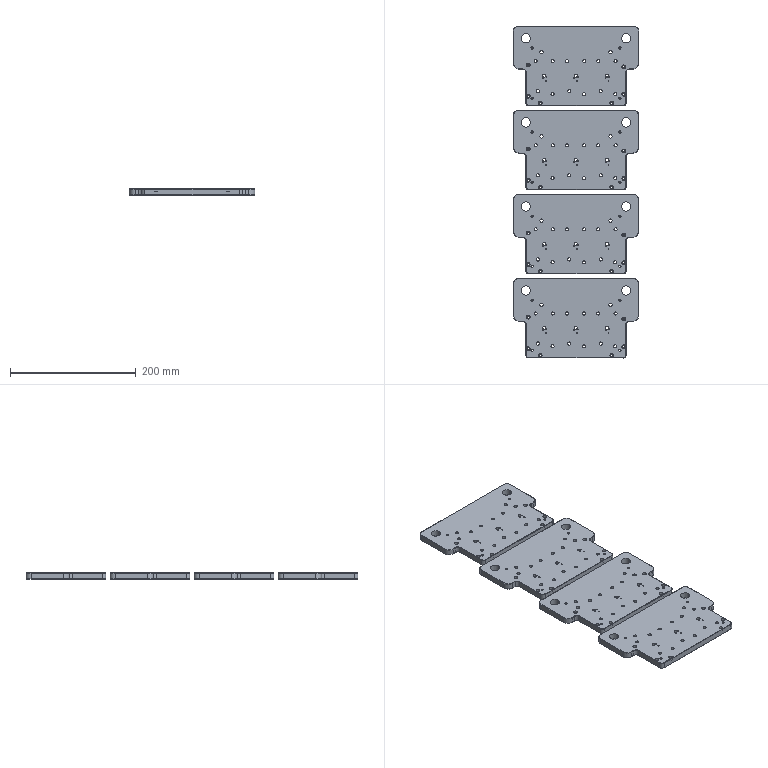NC program | NX | posted with a generic post | part box 200 x 529 x 10 mm
Lines 1 to 1503 of 1801, first 1182 of 1477 lines:
N10 G17 G21 G94 G90
(DRILLING_COPY , TOOL : D4A45)
N12 T02 M6
N14 G54
N16 G17 G0 G90 X80. Y44. S5000 M3
N18 G43 Z30. H2
N20 G94 G81 G98 Z-0.6 F250. R3.
N22 X70. Y28.5
N24 X55. Y21.5
N26 X64.397 Y7.41
N28 X76. Y1.5
N30 X60.727 Y-40.475
N32 X76. Y-48.5
N34 X70. Y-51.5
N36 X57. Y-59.5
N38 X37.379 Y-45.039
N40 X48.194 Y-24.555
N42 Y-23.158
N44 X52.858 Y-18.927
N46 X50.608 Y-15.627
N48 X47.178 Y-17.697
N50 X36.956 Y7.4
N52 X14.397 Y7.41
N54 X-13.044 Y7.4
N56 X-2.822 Y-17.697
N58 X0.608 Y-15.627
N60 X2.858 Y-18.927
N62 X-1.806 Y-23.158
N64 Y-24.555
N66 X10.727 Y-40.475
N68 X-12.621 Y-45.039
N70 X-39.273 Y-40.475
N72 X-57. Y-59.5
N74 X-70. Y-51.5
N76 X-76. Y-45.5
N78 X-62.621 Y-45.039
N80 X-51.806 Y-24.555
N82 Y-23.158
N84 X-47.142 Y-18.927
N86 X-49.392 Y-15.627
N88 X-52.822 Y-17.697
N90 X-76. Y-1.5
N92 X-63.044 Y7.4
N94 X-35.603 Y7.41
N96 X-55. Y21.5
N98 X-70. Y28.5
N100 X-80. Y44.
N102 G80
N104 G0 X-80. Y44. Z30.
N106 M5
(DRILLING_COPY_COPY_COPY_COPY_COPY_COPY , TOOL : 1.7ZT)
N108 T17 M6
N110 G54
N112 G17 G0 G90 X-47.142 Y-18.927 S2000 M3
N114 G43 Z30. H17
N116 G94 G83 G98 Z-12.011 F120. Q2. R3.
N118 X2.858
N120 X52.858
N122 G80
N124 G0 X52.858 Y-18.927 Z30.
N126 M5
(DRILLING_COPY_COPY_COPY_COPY_COPY_COPY_COPY , TOOL : 0.97ZT)
N128 T19 M6
N130 G54
N132 G17 G0 G90 X-52.822 Y-17.697 S2000 M3
N134 G43 Z30. H19
N136 G94 G83 G98 Z-11.791 F100. Q2. R3.
N138 X-51.806 Y-23.158
N140 Y-24.555
N142 X-2.822 Y-17.697
N144 X-1.806 Y-23.158
N146 Y-24.555
N148 X47.178 Y-17.697
N150 X48.194 Y-23.158
N152 Y-24.555
N154 G80
N156 G0 X48.194 Y-24.555 Z30.
N158 M5
(DRILLING_COPY_COPY_COPY_COPY_COPY , TOOL : 3.5ZT)
N160 T15 M6
N162 G54
N164 G17 G0 G90 X76. Y1.5 S1910 M3
N166 G43 Z30. H15
N168 G94 G83 G98 Z-8.552 F180. Q2. R3.
N170 Y-48.5
N172 X57. Y-59.5
N174 X-57.
N176 X-76. Y-45.5
N178 Y-1.5
N180 G80
N182 G0 X-76. Y-1.5 Z30.
(DRILLING_COPY_COPY_COPY_COPY_COPY_COPY_1 , TOOL : 3.5ZT)
N184 X-70. Y28.5
N186 G83 Z-12.552 F180. Q2. R3.
N188 Y-51.5
N190 X70.
N192 Y28.5
N194 G80
N196 G0 X70. Y28.5 Z30.
(DRILLING_COPY_COPY_COPY_COPY_COPY_COPY_1_COPY , TOOL : 3.5ZT)
N198 X-12.621 Y-45.039
N200 G83 Z-12.552 F180. Q2. R3.
N202 X10.727 Y-40.475
N204 X37.379 Y-45.039
N206 X60.727 Y-40.475
N208 X50.608 Y-15.627
N210 X64.397 Y7.41
N212 X55. Y21.5
N214 X36.956 Y7.4
N216 X14.397 Y7.41
N218 X0.608 Y-15.627
N220 X-13.044 Y7.4
N222 X-35.603 Y7.41
N224 X-55. Y21.5
N226 X-63.044 Y7.4
N228 X-49.392 Y-15.627
N230 X-39.273 Y-40.475
N232 X-62.621 Y-45.039
N234 G80
N236 G0 X-62.621 Y-45.039 Z30.
N238 M5
(HOLE_MILLING_COPY , TOOL : D4)
N240 T04 M6
N242 G54
N244 G17 G0 G90 X-70. Y28.5 S9500 M3
N246 G43 Z30. H4
N248 Z0.5
N250 G94 G3 X-70.625 Y29.125 R0.625 F2200.
N252 X-71.25 Y28.5 R0.625
N254 X-71.25 Y28.5 Z0.1 I1.25 J0.
N256 X-71.25 Y28.5 Z-0.3 I1.25 J0.
N258 X-71.25 Y28.5 Z-0.7 I1.25 J0.
N260 X-71.25 Y28.5 Z-1.1 I1.25 J0.
N262 X-71.25 Y28.5 Z-1.5 I1.25 J0.
N264 X-71.25 Y28.5 Z-1.9 I1.25 J0.
N266 X-71.25 Y28.5 Z-2.3 I1.25 J0.
N268 X-71.25 Y28.5 Z-2.7 I1.25 J0.
N270 X-71.25 Y28.5 Z-3.1 I1.25 J0.
N272 X-71.25 Y28.5 Z-3.5 I1.25 J0.
N274 X-71.25 Y28.5 Z-3.9 I1.25 J0.
N276 X-70. Y27.25 Z-4. R1.25
N278 X-68.75 Y28.5 R1.25
N280 X-70. Y27.25 R-1.25
N282 X-69.375 Y27.875 R0.625
N284 X-70. Y28.5 R0.625
N286 G0 Z30.
N288 X-55. Y21.5
N290 Z0.5
N292 G3 X-55.5 Y22. R0.5
N294 X-56. Y21.5 R0.5
N296 X-56. Y21.5 Z0.1 I1. J0.
N298 X-56. Y21.5 Z-0.3 I1. J0.
N300 X-56. Y21.5 Z-0.7 I1. J0.
N302 X-56. Y21.5 Z-1.1 I1. J0.
N304 X-56. Y21.5 Z-1.5 I1. J0.
N306 X-56. Y21.5 Z-1.9 I1. J0.
N308 X-55. Y20.5 Z-2. R1.
N310 X-54. Y21.5 R1.
N312 X-55. Y20.5 R-1.
N314 X-54.5 Y21. R0.5
N316 X-55. Y21.5 R0.5
N318 G0 Z30.
N320 X-70. Y-51.5
N322 Z0.5
N324 G3 X-70.625 Y-50.875 R0.625
N326 X-71.25 Y-51.5 R0.625
N328 X-71.25 Y-51.5 Z0.1 I1.25 J0.
N330 X-71.25 Y-51.5 Z-0.3 I1.25 J0.
N332 X-71.25 Y-51.5 Z-0.7 I1.25 J0.
N334 X-71.25 Y-51.5 Z-1.1 I1.25 J0.
N336 X-71.25 Y-51.5 Z-1.5 I1.25 J0.
N338 X-71.25 Y-51.5 Z-1.9 I1.25 J0.
N340 X-71.25 Y-51.5 Z-2.3 I1.25 J0.
N342 X-71.25 Y-51.5 Z-2.7 I1.25 J0.
N344 X-71.25 Y-51.5 Z-3.1 I1.25 J0.
N346 X-71.25 Y-51.5 Z-3.5 I1.25 J0.
N348 X-71.25 Y-51.5 Z-3.9 I1.25 J0.
N350 X-70. Y-52.75 Z-4. R1.25
N352 X-68.75 Y-51.5 R1.25
N354 X-70. Y-52.75 R-1.25
N356 X-69.375 Y-52.125 R0.625
N358 X-70. Y-51.5 R0.625
N360 G0 Z30.
N362 X70.
N364 Z0.5
N366 G3 X69.375 Y-50.875 R0.625
N368 X68.75 Y-51.5 R0.625
N370 X68.75 Y-51.5 Z0.1 I1.25 J0.
N372 X68.75 Y-51.5 Z-0.3 I1.25 J0.
N374 X68.75 Y-51.5 Z-0.7 I1.25 J0.
N376 X68.75 Y-51.5 Z-1.1 I1.25 J0.
N378 X68.75 Y-51.5 Z-1.5 I1.25 J0.
N380 X68.75 Y-51.5 Z-1.9 I1.25 J0.
N382 X68.75 Y-51.5 Z-2.3 I1.25 J0.
N384 X68.75 Y-51.5 Z-2.7 I1.25 J0.
N386 X68.75 Y-51.5 Z-3.1 I1.25 J0.
N388 X68.75 Y-51.5 Z-3.5 I1.25 J0.
N390 X68.75 Y-51.5 Z-3.9 I1.25 J0.
N392 X70. Y-52.75 Z-4. R1.25
N394 X71.25 Y-51.5 R1.25
N396 X70. Y-52.75 R-1.25
N398 X70.625 Y-52.125 R0.625
N400 X70. Y-51.5 R0.625
N402 G0 Z30.
N404 Y28.5
N406 Z0.5
N408 G3 X69.375 Y29.125 R0.625
N410 X68.75 Y28.5 R0.625
N412 X68.75 Y28.5 Z0.1 I1.25 J0.
N414 X68.75 Y28.5 Z-0.3 I1.25 J0.
N416 X68.75 Y28.5 Z-0.7 I1.25 J0.
N418 X68.75 Y28.5 Z-1.1 I1.25 J0.
N420 X68.75 Y28.5 Z-1.5 I1.25 J0.
N422 X68.75 Y28.5 Z-1.9 I1.25 J0.
N424 X68.75 Y28.5 Z-2.3 I1.25 J0.
N426 X68.75 Y28.5 Z-2.7 I1.25 J0.
N428 X68.75 Y28.5 Z-3.1 I1.25 J0.
N430 X68.75 Y28.5 Z-3.5 I1.25 J0.
N432 X68.75 Y28.5 Z-3.9 I1.25 J0.
N434 X70. Y27.25 Z-4. R1.25
N436 X71.25 Y28.5 R1.25
N438 X70. Y27.25 R-1.25
N440 X70.625 Y27.875 R0.625
N442 X70. Y28.5 R0.625
N444 G0 Z30.
N446 X55. Y21.5
N448 Z0.5
N450 G3 X54.5 Y22. R0.5
N452 X54. Y21.5 R0.5
N454 X54. Y21.5 Z0.1 I1. J0.
N456 X54. Y21.5 Z-0.3 I1. J0.
N458 X54. Y21.5 Z-0.7 I1. J0.
N460 X54. Y21.5 Z-1.1 I1. J0.
N462 X54. Y21.5 Z-1.5 I1. J0.
N464 X54. Y21.5 Z-1.9 I1. J0.
N466 X55. Y20.5 Z-2. R1.
N468 X56. Y21.5 R1.
N470 X55. Y20.5 R-1.
N472 X55.5 Y21. R0.5
N474 X55. Y21.5 R0.5
N476 G0 Z30.
N478 M5
(HOLE_MILLING_1 , TOOL : D6)
N480 T06 M6
N482 G54
N484 G17 G0 G90 X-80. Y44. S9500 M3
N486 G43 Z30. H6
N488 Z0.5
N490 G94 G3 X-81.1 Y45.1 R1.1 F2200.
N492 X-82.2 Y44. R1.1
N494 X-82.2 Y44. Z0. I2.2 J0.
N496 X-82.2 Y44. Z-0.5 I2.2 J0.
N498 X-82.2 Y44. Z-1. I2.2 J0.
N500 X-82.2 Y44. Z-1.5 I2.2 J0.
N502 X-82.2 Y44. Z-2. I2.2 J0.
N504 X-82.2 Y44. Z-2.5 I2.2 J0.
N506 X-82.2 Y44. Z-3. I2.2 J0.
N508 X-82.2 Y44. Z-3.5 I2.2 J0.
N510 X-82.2 Y44. Z-4. I2.2 J0.
N512 X-82.2 Y44. Z-4.5 I2.2 J0.
N514 X-82.2 Y44. Z-5. I2.2 J0.
N516 X-82.2 Y44. Z-5.5 I2.2 J0.
N518 X-82.2 Y44. Z-6. I2.2 J0.
N520 X-82.2 Y44. Z-6.5 I2.2 J0.
N522 X-82.2 Y44. Z-7. I2.2 J0.
N524 X-82.2 Y44. Z-7.5 I2.2 J0.
N526 X-82.2 Y44. Z-8. I2.2 J0.
N528 X-82.2 Y44. Z-8.5 I2.2 J0.
N530 X-82.2 Y44. Z-9. I2.2 J0.
N532 X-82.2 Y44. Z-9.5 I2.2 J0.
N534 X-82.2 Y44. Z-10. I2.2 J0.
N536 X-80. Y41.8 R2.2
N538 X-82.2 Y44. R-2.2
N540 X-81.1 Y42.9 R1.1
N542 X-80. Y44. R1.1
N544 G0 Z0.5
N546 G3 X-82.2 Y46.2 R2.2
N548 X-84.4 Y44. R2.2
N550 X-84.4 Y44. Z0. I4.4 J0.
N552 X-84.4 Y44. Z-0.5 I4.4 J0.
N554 X-84.4 Y44. Z-1. I4.4 J0.
N556 X-84.4 Y44. Z-1.5 I4.4 J0.
N558 X-84.4 Y44. Z-2. I4.4 J0.
N560 X-84.4 Y44. Z-2.5 I4.4 J0.
N562 X-84.4 Y44. Z-3. I4.4 J0.
N564 X-84.4 Y44. Z-3.5 I4.4 J0.
N566 X-84.4 Y44. Z-4. I4.4 J0.
N568 X-84.4 Y44. Z-4.5 I4.4 J0.
N570 X-84.4 Y44. Z-5. I4.4 J0.
N572 X-84.4 Y44. Z-5.5 I4.4 J0.
N574 X-84.4 Y44. Z-6. I4.4 J0.
N576 X-84.4 Y44. Z-6.5 I4.4 J0.
N578 X-84.4 Y44. Z-7. I4.4 J0.
N580 X-84.4 Y44. Z-7.5 I4.4 J0.
N582 X-84.4 Y44. Z-8. I4.4 J0.
N584 X-84.4 Y44. Z-8.5 I4.4 J0.
N586 X-84.4 Y44. Z-9. I4.4 J0.
N588 X-84.4 Y44. Z-9.5 I4.4 J0.
N590 X-84.4 Y44. Z-10. I4.4 J0.
N592 X-80. Y39.6 R4.4
N594 X-84.4 Y44. R-4.4
N596 X-82.2 Y41.8 R2.2
N598 X-80. Y44. R2.2
N600 G0 Z30.
N602 X80.
N604 Z0.5
N606 G3 X78.9 Y45.1 R1.1
N608 X77.8 Y44. R1.1
N610 X77.8 Y44. Z0. I2.2 J0.
N612 X77.8 Y44. Z-0.5 I2.2 J0.
N614 X77.8 Y44. Z-1. I2.2 J0.
N616 X77.8 Y44. Z-1.5 I2.2 J0.
N618 X77.8 Y44. Z-2. I2.2 J0.
N620 X77.8 Y44. Z-2.5 I2.2 J0.
N622 X77.8 Y44. Z-3. I2.2 J0.
N624 X77.8 Y44. Z-3.5 I2.2 J0.
N626 X77.8 Y44. Z-4. I2.2 J0.
N628 X77.8 Y44. Z-4.5 I2.2 J0.
N630 X77.8 Y44. Z-5. I2.2 J0.
N632 X77.8 Y44. Z-5.5 I2.2 J0.
N634 X77.8 Y44. Z-6. I2.2 J0.
N636 X77.8 Y44. Z-6.5 I2.2 J0.
N638 X77.8 Y44. Z-7. I2.2 J0.
N640 X77.8 Y44. Z-7.5 I2.2 J0.
N642 X77.8 Y44. Z-8. I2.2 J0.
N644 X77.8 Y44. Z-8.5 I2.2 J0.
N646 X77.8 Y44. Z-9. I2.2 J0.
N648 X77.8 Y44. Z-9.5 I2.2 J0.
N650 X77.8 Y44. Z-10. I2.2 J0.
N652 X80. Y41.8 R2.2
N654 X77.8 Y44. R-2.2
N656 X78.9 Y42.9 R1.1
N658 X80. Y44. R1.1
N660 G0 Z0.5
N662 G3 X77.8 Y46.2 R2.2
N664 X75.6 Y44. R2.2
N666 X75.6 Y44. Z0. I4.4 J0.
N668 X75.6 Y44. Z-0.5 I4.4 J0.
N670 X75.6 Y44. Z-1. I4.4 J0.
N672 X75.6 Y44. Z-1.5 I4.4 J0.
N674 X75.6 Y44. Z-2. I4.4 J0.
N676 X75.6 Y44. Z-2.5 I4.4 J0.
N678 X75.6 Y44. Z-3. I4.4 J0.
N680 X75.6 Y44. Z-3.5 I4.4 J0.
N682 X75.6 Y44. Z-4. I4.4 J0.
N684 X75.6 Y44. Z-4.5 I4.4 J0.
N686 X75.6 Y44. Z-5. I4.4 J0.
N688 X75.6 Y44. Z-5.5 I4.4 J0.
N690 X75.6 Y44. Z-6. I4.4 J0.
N692 X75.6 Y44. Z-6.5 I4.4 J0.
N694 X75.6 Y44. Z-7. I4.4 J0.
N696 X75.6 Y44. Z-7.5 I4.4 J0.
N698 X75.6 Y44. Z-8. I4.4 J0.
N700 X75.6 Y44. Z-8.5 I4.4 J0.
N702 X75.6 Y44. Z-9. I4.4 J0.
N704 X75.6 Y44. Z-9.5 I4.4 J0.
N706 X75.6 Y44. Z-10. I4.4 J0.
N708 X80. Y39.6 R4.4
N710 X75.6 Y44. R-4.4
N712 X77.8 Y41.8 R2.2
N714 X80. Y44. R2.2
N716 G0 Z30.
N718 M5
(HOLE_MILLING_COPY_COPY , TOOL : D3)
N720 T03 M6
N722 G54
N724 G17 G0 G90 X-63.044 Y7.4 S9500 M3
N726 G43 Z30. H3
N728 Z0.5
N730 G94 G3 X-63.494 Y7.85 R0.45 F1000.
N732 X-63.944 Y7.4 R0.45
N734 X-63.944 Y7.4 Z0.2 I0.9 J0.
N736 X-63.944 Y7.4 Z-0.1 I0.9 J0.
N738 X-63.944 Y7.4 Z-0.4 I0.9 J0.
N740 X-63.944 Y7.4 Z-0.7 I0.9 J0.
N742 X-63.944 Y7.4 Z-1. I0.9 J0.
N744 X-63.944 Y7.4 Z-1.3 I0.9 J0.
N746 X-63.944 Y7.4 Z-1.6 I0.9 J0.
N748 X-63.944 Y7.4 Z-1.9 I0.9 J0.
N750 X-63.944 Y7.4 Z-2.2 I0.9 J0.
N752 X-63.944 Y7.4 Z-2.5 I0.9 J0.
N754 X-63.944 Y7.4 Z-2.8 I0.9 J0.
N756 X-63.944 Y7.4 Z-3.1 I0.9 J0.
N758 X-63.944 Y7.4 Z-3.4 I0.9 J0.
N760 X-63.944 Y7.4 Z-3.7 I0.9 J0.
N762 X-63.944 Y7.4 Z-4. I0.9 J0.
N764 X-63.944 Y7.4 Z-4.3 I0.9 J0.
N766 X-63.944 Y7.4 Z-4.6 I0.9 J0.
N768 X-63.944 Y7.4 Z-4.9 I0.9 J0.
N770 X-63.944 Y7.4 Z-5.2 I0.9 J0.
N772 X-63.944 Y7.4 Z-5.5 I0.9 J0.
N774 X-63.944 Y7.4 Z-5.8 I0.9 J0.
N776 X-63.944 Y7.4 Z-6.1 I0.9 J0.
N778 X-63.944 Y7.4 Z-6.4 I0.9 J0.
N780 X-63.944 Y7.4 Z-6.7 I0.9 J0.
N782 X-63.944 Y7.4 Z-7. I0.9 J0.
N784 X-63.944 Y7.4 Z-7.3 I0.9 J0.
N786 X-63.944 Y7.4 Z-7.6 I0.9 J0.
N788 X-63.944 Y7.4 Z-7.9 I0.9 J0.
N790 X-63.944 Y7.4 Z-8.2 I0.9 J0.
N792 X-63.944 Y7.4 Z-8.5 I0.9 J0.
N794 X-63.944 Y7.4 Z-8.8 I0.9 J0.
N796 X-63.944 Y7.4 Z-9.1 I0.9 J0.
N798 X-63.944 Y7.4 Z-9.4 I0.9 J0.
N800 X-63.944 Y7.4 Z-9.7 I0.9 J0.
N802 X-63.944 Y7.4 Z-10. I0.9 J0.
N804 X-63.044 Y6.5 R0.9
N806 X-63.944 Y7.4 R-0.9
N808 X-63.494 Y6.95 R0.45
N810 X-63.044 Y7.4 R0.45
N812 G0 Z30.
N814 X-49.392 Y-15.627
N816 Z0.5
N818 G3 X-49.842 Y-15.177 R0.45
N820 X-50.292 Y-15.627 R0.45
N822 X-50.292 Y-15.627 Z0.2 I0.9 J0.
N824 X-50.292 Y-15.627 Z-0.1 I0.9 J0.
N826 X-50.292 Y-15.627 Z-0.4 I0.9 J0.
N828 X-50.292 Y-15.627 Z-0.7 I0.9 J0.
N830 X-50.292 Y-15.627 Z-1. I0.9 J0.
N832 X-50.292 Y-15.627 Z-1.3 I0.9 J0.
N834 X-50.292 Y-15.627 Z-1.6 I0.9 J0.
N836 X-50.292 Y-15.627 Z-1.9 I0.9 J0.
N838 X-50.292 Y-15.627 Z-2.2 I0.9 J0.
N840 X-50.292 Y-15.627 Z-2.5 I0.9 J0.
N842 X-50.292 Y-15.627 Z-2.8 I0.9 J0.
N844 X-50.292 Y-15.627 Z-3.1 I0.9 J0.
N846 X-50.292 Y-15.627 Z-3.4 I0.9 J0.
N848 X-50.292 Y-15.627 Z-3.7 I0.9 J0.
N850 X-50.292 Y-15.627 Z-4. I0.9 J0.
N852 X-50.292 Y-15.627 Z-4.3 I0.9 J0.
N854 X-50.292 Y-15.627 Z-4.6 I0.9 J0.
N856 X-50.292 Y-15.627 Z-4.9 I0.9 J0.
N858 X-50.292 Y-15.627 Z-5.2 I0.9 J0.
N860 X-50.292 Y-15.627 Z-5.5 I0.9 J0.
N862 X-50.292 Y-15.627 Z-5.8 I0.9 J0.
N864 X-50.292 Y-15.627 Z-6.1 I0.9 J0.
N866 X-50.292 Y-15.627 Z-6.4 I0.9 J0.
N868 X-50.292 Y-15.627 Z-6.7 I0.9 J0.
N870 X-50.292 Y-15.627 Z-7. I0.9 J0.
N872 X-50.292 Y-15.627 Z-7.3 I0.9 J0.
N874 X-50.292 Y-15.627 Z-7.6 I0.9 J0.
N876 X-50.292 Y-15.627 Z-7.9 I0.9 J0.
N878 X-50.292 Y-15.627 Z-8.2 I0.9 J0.
N880 X-50.292 Y-15.627 Z-8.5 I0.9 J0.
N882 X-50.292 Y-15.627 Z-8.8 I0.9 J0.
N884 X-50.292 Y-15.627 Z-9.1 I0.9 J0.
N886 X-50.292 Y-15.627 Z-9.4 I0.9 J0.
N888 X-50.292 Y-15.627 Z-9.7 I0.9 J0.
N890 X-50.292 Y-15.627 Z-10. I0.9 J0.
N892 X-49.392 Y-16.527 R0.9
N894 X-50.292 Y-15.627 R-0.9
N896 X-49.842 Y-16.077 R0.45
N898 X-49.392 Y-15.627 R0.45
N900 G0 Z30.
N902 X-35.603 Y7.41
N904 Z0.5
N906 G3 X-36.053 Y7.86 R0.45
N908 X-36.503 Y7.41 R0.45
N910 X-36.503 Y7.41 Z0.2 I0.9 J0.
N912 X-36.503 Y7.41 Z-0.1 I0.9 J0.
N914 X-36.503 Y7.41 Z-0.4 I0.9 J0.
N916 X-36.503 Y7.41 Z-0.7 I0.9 J0.
N918 X-36.503 Y7.41 Z-1. I0.9 J0.
N920 X-36.503 Y7.41 Z-1.3 I0.9 J0.
N922 X-36.503 Y7.41 Z-1.6 I0.9 J0.
N924 X-36.503 Y7.41 Z-1.9 I0.9 J0.
N926 X-36.503 Y7.41 Z-2.2 I0.9 J0.
N928 X-36.503 Y7.41 Z-2.5 I0.9 J0.
N930 X-36.503 Y7.41 Z-2.8 I0.9 J0.
N932 X-36.503 Y7.41 Z-3.1 I0.9 J0.
N934 X-36.503 Y7.41 Z-3.4 I0.9 J0.
N936 X-36.503 Y7.41 Z-3.7 I0.9 J0.
N938 X-36.503 Y7.41 Z-4. I0.9 J0.
N940 X-36.503 Y7.41 Z-4.3 I0.9 J0.
N942 X-36.503 Y7.41 Z-4.6 I0.9 J0.
N944 X-36.503 Y7.41 Z-4.9 I0.9 J0.
N946 X-36.503 Y7.41 Z-5.2 I0.9 J0.
N948 X-36.503 Y7.41 Z-5.5 I0.9 J0.
N950 X-36.503 Y7.41 Z-5.8 I0.9 J0.
N952 X-36.503 Y7.41 Z-6.1 I0.9 J0.
N954 X-36.503 Y7.41 Z-6.4 I0.9 J0.
N956 X-36.503 Y7.41 Z-6.7 I0.9 J0.
N958 X-36.503 Y7.41 Z-7. I0.9 J0.
N960 X-36.503 Y7.41 Z-7.3 I0.9 J0.
N962 X-36.503 Y7.41 Z-7.6 I0.9 J0.
N964 X-36.503 Y7.41 Z-7.9 I0.9 J0.
N966 X-36.503 Y7.41 Z-8.2 I0.9 J0.
N968 X-36.503 Y7.41 Z-8.5 I0.9 J0.
N970 X-36.503 Y7.41 Z-8.8 I0.9 J0.
N972 X-36.503 Y7.41 Z-9.1 I0.9 J0.
N974 X-36.503 Y7.41 Z-9.4 I0.9 J0.
N976 X-36.503 Y7.41 Z-9.7 I0.9 J0.
N978 X-36.503 Y7.41 Z-10. I0.9 J0.
N980 X-35.603 Y6.51 R0.9
N982 X-36.503 Y7.41 R-0.9
N984 X-36.053 Y6.96 R0.45
N986 X-35.603 Y7.41 R0.45
N988 G0 Z30.
N990 X-13.044 Y7.4
N992 Z0.5
N994 G3 X-13.494 Y7.85 R0.45
N996 X-13.944 Y7.4 R0.45
N998 X-13.944 Y7.4 Z0.2 I0.9 J0.
N1000 X-13.944 Y7.4 Z-0.1 I0.9 J0.
N1002 X-13.944 Y7.4 Z-0.4 I0.9 J0.
N1004 X-13.944 Y7.4 Z-0.7 I0.9 J0.
N1006 X-13.944 Y7.4 Z-1. I0.9 J0.
N1008 X-13.944 Y7.4 Z-1.3 I0.9 J0.
N1010 X-13.944 Y7.4 Z-1.6 I0.9 J0.
N1012 X-13.944 Y7.4 Z-1.9 I0.9 J0.
N1014 X-13.944 Y7.4 Z-2.2 I0.9 J0.
N1016 X-13.944 Y7.4 Z-2.5 I0.9 J0.
N1018 X-13.944 Y7.4 Z-2.8 I0.9 J0.
N1020 X-13.944 Y7.4 Z-3.1 I0.9 J0.
N1022 X-13.944 Y7.4 Z-3.4 I0.9 J0.
N1024 X-13.944 Y7.4 Z-3.7 I0.9 J0.
N1026 X-13.944 Y7.4 Z-4. I0.9 J0.
N1028 X-13.944 Y7.4 Z-4.3 I0.9 J0.
N1030 X-13.944 Y7.4 Z-4.6 I0.9 J0.
N1032 X-13.944 Y7.4 Z-4.9 I0.9 J0.
N1034 X-13.944 Y7.4 Z-5.2 I0.9 J0.
N1036 X-13.944 Y7.4 Z-5.5 I0.9 J0.
N1038 X-13.944 Y7.4 Z-5.8 I0.9 J0.
N1040 X-13.944 Y7.4 Z-6.1 I0.9 J0.
N1042 X-13.944 Y7.4 Z-6.4 I0.9 J0.
N1044 X-13.944 Y7.4 Z-6.7 I0.9 J0.
N1046 X-13.944 Y7.4 Z-7. I0.9 J0.
N1048 X-13.944 Y7.4 Z-7.3 I0.9 J0.
N1050 X-13.944 Y7.4 Z-7.6 I0.9 J0.
N1052 X-13.944 Y7.4 Z-7.9 I0.9 J0.
N1054 X-13.944 Y7.4 Z-8.2 I0.9 J0.
N1056 X-13.944 Y7.4 Z-8.5 I0.9 J0.
N1058 X-13.944 Y7.4 Z-8.8 I0.9 J0.
N1060 X-13.944 Y7.4 Z-9.1 I0.9 J0.
N1062 X-13.944 Y7.4 Z-9.4 I0.9 J0.
N1064 X-13.944 Y7.4 Z-9.7 I0.9 J0.
N1066 X-13.944 Y7.4 Z-10. I0.9 J0.
N1068 X-13.044 Y6.5 R0.9
N1070 X-13.944 Y7.4 R-0.9
N1072 X-13.494 Y6.95 R0.45
N1074 X-13.044 Y7.4 R0.45
N1076 G0 Z30.
N1078 X0.608 Y-15.627
N1080 Z0.5
N1082 G3 X0.158 Y-15.177 R0.45
N1084 X-0.292 Y-15.627 R0.45
N1086 X-0.292 Y-15.627 Z0.2 I0.9 J0.
N1088 X-0.292 Y-15.627 Z-0.1 I0.9 J0.
N1090 X-0.292 Y-15.627 Z-0.4 I0.9 J0.
N1092 X-0.292 Y-15.627 Z-0.7 I0.9 J0.
N1094 X-0.292 Y-15.627 Z-1. I0.9 J0.
N1096 X-0.292 Y-15.627 Z-1.3 I0.9 J0.
N1098 X-0.292 Y-15.627 Z-1.6 I0.9 J0.
N1100 X-0.292 Y-15.627 Z-1.9 I0.9 J0.
N1102 X-0.292 Y-15.627 Z-2.2 I0.9 J0.
N1104 X-0.292 Y-15.627 Z-2.5 I0.9 J0.
N1106 X-0.292 Y-15.627 Z-2.8 I0.9 J0.
N1108 X-0.292 Y-15.627 Z-3.1 I0.9 J0.
N1110 X-0.292 Y-15.627 Z-3.4 I0.9 J0.
N1112 X-0.292 Y-15.627 Z-3.7 I0.9 J0.
N1114 X-0.292 Y-15.627 Z-4. I0.9 J0.
N1116 X-0.292 Y-15.627 Z-4.3 I0.9 J0.
N1118 X-0.292 Y-15.627 Z-4.6 I0.9 J0.
N1120 X-0.292 Y-15.627 Z-4.9 I0.9 J0.
N1122 X-0.292 Y-15.627 Z-5.2 I0.9 J0.
N1124 X-0.292 Y-15.627 Z-5.5 I0.9 J0.
N1126 X-0.292 Y-15.627 Z-5.8 I0.9 J0.
N1128 X-0.292 Y-15.627 Z-6.1 I0.9 J0.
N1130 X-0.292 Y-15.627 Z-6.4 I0.9 J0.
N1132 X-0.292 Y-15.627 Z-6.7 I0.9 J0.
N1134 X-0.292 Y-15.627 Z-7. I0.9 J0.
N1136 X-0.292 Y-15.627 Z-7.3 I0.9 J0.
N1138 X-0.292 Y-15.627 Z-7.6 I0.9 J0.
N1140 X-0.292 Y-15.627 Z-7.9 I0.9 J0.
N1142 X-0.292 Y-15.627 Z-8.2 I0.9 J0.
N1144 X-0.292 Y-15.627 Z-8.5 I0.9 J0.
N1146 X-0.292 Y-15.627 Z-8.8 I0.9 J0.
N1148 X-0.292 Y-15.627 Z-9.1 I0.9 J0.
N1150 X-0.292 Y-15.627 Z-9.4 I0.9 J0.
N1152 X-0.292 Y-15.627 Z-9.7 I0.9 J0.
N1154 X-0.292 Y-15.627 Z-10. I0.9 J0.
N1156 X0.608 Y-16.527 R0.9
N1158 X-0.292 Y-15.627 R-0.9
N1160 X0.158 Y-16.077 R0.45
N1162 X0.608 Y-15.627 R0.45
N1164 G0 Z30.
N1166 X14.397 Y7.41
N1168 Z0.5
N1170 G3 X13.947 Y7.86 R0.45
N1172 X13.497 Y7.41 R0.45
N1174 X13.497 Y7.41 Z0.2 I0.9 J0.
N1176 X13.497 Y7.41 Z-0.1 I0.9 J0.
N1178 X13.497 Y7.41 Z-0.4 I0.9 J0.
N1180 X13.497 Y7.41 Z-0.7 I0.9 J0.
N1182 X13.497 Y7.41 Z-1. I0.9 J0.
N1184 X13.497 Y7.41 Z-1.3 I0.9 J0.
N1186 X13.497 Y7.41 Z-1.6 I0.9 J0.
N1188 X13.497 Y7.41 Z-1.9 I0.9 J0.
N1190 X13.497 Y7.41 Z-2.2 I0.9 J0.
N1192 X13.497 Y7.41 Z-2.5 I0.9 J0.
N1194 X13.497 Y7.41 Z-2.8 I0.9 J0.
N1196 X13.497 Y7.41 Z-3.1 I0.9 J0.
N1198 X13.497 Y7.41 Z-3.4 I0.9 J0.
N1200 X13.497 Y7.41 Z-3.7 I0.9 J0.
N1202 X13.497 Y7.41 Z-4. I0.9 J0.
N1204 X13.497 Y7.41 Z-4.3 I0.9 J0.
N1206 X13.497 Y7.41 Z-4.6 I0.9 J0.
N1208 X13.497 Y7.41 Z-4.9 I0.9 J0.
N1210 X13.497 Y7.41 Z-5.2 I0.9 J0.
N1212 X13.497 Y7.41 Z-5.5 I0.9 J0.
N1214 X13.497 Y7.41 Z-5.8 I0.9 J0.
N1216 X13.497 Y7.41 Z-6.1 I0.9 J0.
N1218 X13.497 Y7.41 Z-6.4 I0.9 J0.
N1220 X13.497 Y7.41 Z-6.7 I0.9 J0.
N1222 X13.497 Y7.41 Z-7. I0.9 J0.
N1224 X13.497 Y7.41 Z-7.3 I0.9 J0.
N1226 X13.497 Y7.41 Z-7.6 I0.9 J0.
N1228 X13.497 Y7.41 Z-7.9 I0.9 J0.
N1230 X13.497 Y7.41 Z-8.2 I0.9 J0.
N1232 X13.497 Y7.41 Z-8.5 I0.9 J0.
N1234 X13.497 Y7.41 Z-8.8 I0.9 J0.
N1236 X13.497 Y7.41 Z-9.1 I0.9 J0.
N1238 X13.497 Y7.41 Z-9.4 I0.9 J0.
N1240 X13.497 Y7.41 Z-9.7 I0.9 J0.
N1242 X13.497 Y7.41 Z-10. I0.9 J0.
N1244 X14.397 Y6.51 R0.9
N1246 X13.497 Y7.41 R-0.9
N1248 X13.947 Y6.96 R0.45
N1250 X14.397 Y7.41 R0.45
N1252 G0 Z30.
N1254 X36.956 Y7.4
N1256 Z0.5
N1258 G3 X36.506 Y7.85 R0.45
N1260 X36.056 Y7.4 R0.45
N1262 X36.056 Y7.4 Z0.2 I0.9 J0.
N1264 X36.056 Y7.4 Z-0.1 I0.9 J0.
N1266 X36.056 Y7.4 Z-0.4 I0.9 J0.
N1268 X36.056 Y7.4 Z-0.7 I0.9 J0.
N1270 X36.056 Y7.4 Z-1. I0.9 J0.
N1272 X36.056 Y7.4 Z-1.3 I0.9 J0.
N1274 X36.056 Y7.4 Z-1.6 I0.9 J0.
N1276 X36.056 Y7.4 Z-1.9 I0.9 J0.
N1278 X36.056 Y7.4 Z-2.2 I0.9 J0.
N1280 X36.056 Y7.4 Z-2.5 I0.9 J0.
N1282 X36.056 Y7.4 Z-2.8 I0.9 J0.
N1284 X36.056 Y7.4 Z-3.1 I0.9 J0.
N1286 X36.056 Y7.4 Z-3.4 I0.9 J0.
N1288 X36.056 Y7.4 Z-3.7 I0.9 J0.
N1290 X36.056 Y7.4 Z-4. I0.9 J0.
N1292 X36.056 Y7.4 Z-4.3 I0.9 J0.
N1294 X36.056 Y7.4 Z-4.6 I0.9 J0.
N1296 X36.056 Y7.4 Z-4.9 I0.9 J0.
N1298 X36.056 Y7.4 Z-5.2 I0.9 J0.
N1300 X36.056 Y7.4 Z-5.5 I0.9 J0.
N1302 X36.056 Y7.4 Z-5.8 I0.9 J0.
N1304 X36.056 Y7.4 Z-6.1 I0.9 J0.
N1306 X36.056 Y7.4 Z-6.4 I0.9 J0.
N1308 X36.056 Y7.4 Z-6.7 I0.9 J0.
N1310 X36.056 Y7.4 Z-7. I0.9 J0.
N1312 X36.056 Y7.4 Z-7.3 I0.9 J0.
N1314 X36.056 Y7.4 Z-7.6 I0.9 J0.
N1316 X36.056 Y7.4 Z-7.9 I0.9 J0.
N1318 X36.056 Y7.4 Z-8.2 I0.9 J0.
N1320 X36.056 Y7.4 Z-8.5 I0.9 J0.
N1322 X36.056 Y7.4 Z-8.8 I0.9 J0.
N1324 X36.056 Y7.4 Z-9.1 I0.9 J0.
N1326 X36.056 Y7.4 Z-9.4 I0.9 J0.
N1328 X36.056 Y7.4 Z-9.7 I0.9 J0.
N1330 X36.056 Y7.4 Z-10. I0.9 J0.
N1332 X36.956 Y6.5 R0.9
N1334 X36.056 Y7.4 R-0.9
N1336 X36.506 Y6.95 R0.45
N1338 X36.956 Y7.4 R0.45
N1340 G0 Z30.
N1342 X64.397 Y7.41
N1344 Z0.5
N1346 G3 X63.947 Y7.86 R0.45
N1348 X63.497 Y7.41 R0.45
N1350 X63.497 Y7.41 Z0.2 I0.9 J0.
N1352 X63.497 Y7.41 Z-0.1 I0.9 J0.
N1354 X63.497 Y7.41 Z-0.4 I0.9 J0.
N1356 X63.497 Y7.41 Z-0.7 I0.9 J0.
N1358 X63.497 Y7.41 Z-1. I0.9 J0.
N1360 X63.497 Y7.41 Z-1.3 I0.9 J0.
N1362 X63.497 Y7.41 Z-1.6 I0.9 J0.
N1364 X63.497 Y7.41 Z-1.9 I0.9 J0.
N1366 X63.497 Y7.41 Z-2.2 I0.9 J0.
N1368 X63.497 Y7.41 Z-2.5 I0.9 J0.
N1370 X63.497 Y7.41 Z-2.8 I0.9 J0.
N1372 X63.497 Y7.41 Z-3.1 I0.9 J0.
N1374 X63.497 Y7.41 Z-3.4 I0.9 J0.
N1376 X63.497 Y7.41 Z-3.7 I0.9 J0.
N1378 X63.497 Y7.41 Z-4. I0.9 J0.
N1380 X63.497 Y7.41 Z-4.3 I0.9 J0.
N1382 X63.497 Y7.41 Z-4.6 I0.9 J0.
N1384 X63.497 Y7.41 Z-4.9 I0.9 J0.
N1386 X63.497 Y7.41 Z-5.2 I0.9 J0.
N1388 X63.497 Y7.41 Z-5.5 I0.9 J0.
N1390 X63.497 Y7.41 Z-5.8 I0.9 J0.
N1392 X63.497 Y7.41 Z-6.1 I0.9 J0.
N1394 X63.497 Y7.41 Z-6.4 I0.9 J0.
N1396 X63.497 Y7.41 Z-6.7 I0.9 J0.
N1398 X63.497 Y7.41 Z-7. I0.9 J0.
N1400 X63.497 Y7.41 Z-7.3 I0.9 J0.
N1402 X63.497 Y7.41 Z-7.6 I0.9 J0.
N1404 X63.497 Y7.41 Z-7.9 I0.9 J0.
N1406 X63.497 Y7.41 Z-8.2 I0.9 J0.
N1408 X63.497 Y7.41 Z-8.5 I0.9 J0.
N1410 X63.497 Y7.41 Z-8.8 I0.9 J0.
N1412 X63.497 Y7.41 Z-9.1 I0.9 J0.
N1414 X63.497 Y7.41 Z-9.4 I0.9 J0.
N1416 X63.497 Y7.41 Z-9.7 I0.9 J0.
N1418 X63.497 Y7.41 Z-10. I0.9 J0.
N1420 X64.397 Y6.51 R0.9
N1422 X63.497 Y7.41 R-0.9
N1424 X63.947 Y6.96 R0.45
N1426 X64.397 Y7.41 R0.45
N1428 G0 Z30.
N1430 X50.608 Y-15.627
N1432 Z0.5
N1434 G3 X50.158 Y-15.177 R0.45
N1436 X49.708 Y-15.627 R0.45
N1438 X49.708 Y-15.627 Z0.2 I0.9 J0.
N1440 X49.708 Y-15.627 Z-0.1 I0.9 J0.
N1442 X49.708 Y-15.627 Z-0.4 I0.9 J0.
N1444 X49.708 Y-15.627 Z-0.7 I0.9 J0.
N1446 X49.708 Y-15.627 Z-1. I0.9 J0.
N1448 X49.708 Y-15.627 Z-1.3 I0.9 J0.
N1450 X49.708 Y-15.627 Z-1.6 I0.9 J0.
N1452 X49.708 Y-15.627 Z-1.9 I0.9 J0.
N1454 X49.708 Y-15.627 Z-2.2 I0.9 J0.
N1456 X49.708 Y-15.627 Z-2.5 I0.9 J0.
N1458 X49.708 Y-15.627 Z-2.8 I0.9 J0.
N1460 X49.708 Y-15.627 Z-3.1 I0.9 J0.
N1462 X49.708 Y-15.627 Z-3.4 I0.9 J0.
N1464 X49.708 Y-15.627 Z-3.7 I0.9 J0.
N1466 X49.708 Y-15.627 Z-4. I0.9 J0.
N1468 X49.708 Y-15.627 Z-4.3 I0.9 J0.
N1470 X49.708 Y-15.627 Z-4.6 I0.9 J0.
N1472 X49.708 Y-15.627 Z-4.9 I0.9 J0.
N1474 X49.708 Y-15.627 Z-5.2 I0.9 J0.
N1476 X49.708 Y-15.627 Z-5.5 I0.9 J0.
N1478 X49.708 Y-15.627 Z-5.8 I0.9 J0.
N1480 X49.708 Y-15.627 Z-6.1 I0.9 J0.
N1482 X49.708 Y-15.627 Z-6.4 I0.9 J0.
N1484 X49.708 Y-15.627 Z-6.7 I0.9 J0.
N1486 X49.708 Y-15.627 Z-7. I0.9 J0.
N1488 X49.708 Y-15.627 Z-7.3 I0.9 J0.
N1490 X49.708 Y-15.627 Z-7.6 I0.9 J0.
N1492 X49.708 Y-15.627 Z-7.9 I0.9 J0.
N1494 X49.708 Y-15.627 Z-8.2 I0.9 J0.
N1496 X49.708 Y-15.627 Z-8.5 I0.9 J0.
N1498 X49.708 Y-15.627 Z-8.8 I0.9 J0.
N1500 X49.708 Y-15.627 Z-9.1 I0.9 J0.
N1502 X49.708 Y-15.627 Z-9.4 I0.9 J0.
N1504 X49.708 Y-15.627 Z-9.7 I0.9 J0.
N1506 X49.708 Y-15.627 Z-10. I0.9 J0.
N1508 X50.608 Y-16.527 R0.9
N1510 X49.708 Y-15.627 R-0.9
N1512 X50.158 Y-16.077 R0.45
N1514 X50.608 Y-15.627 R0.45
N1516 G0 Z30.
N1518 X60.727 Y-40.475
N1520 Z0.5
N1522 G3 X60.277 Y-40.025 R0.45
N1524 X59.827 Y-40.475 R0.45
N1526 X59.827 Y-40.475 Z0.2 I0.9 J0.
N1528 X59.827 Y-40.475 Z-0.1 I0.9 J0.
N1530 X59.827 Y-40.475 Z-0.4 I0.9 J0.
N1532 X59.827 Y-40.475 Z-0.7 I0.9 J0.
N1534 X59.827 Y-40.475 Z-1. I0.9 J0.
N1536 X59.827 Y-40.475 Z-1.3 I0.9 J0.
N1538 X59.827 Y-40.475 Z-1.6 I0.9 J0.
N1540 X59.827 Y-40.475 Z-1.9 I0.9 J0.
N1542 X59.827 Y-40.475 Z-2.2 I0.9 J0.
N1544 X59.827 Y-40.475 Z-2.5 I0.9 J0.
N1546 X59.827 Y-40.475 Z-2.8 I0.9 J0.
N1548 X59.827 Y-40.475 Z-3.1 I0.9 J0.
N1550 X59.827 Y-40.475 Z-3.4 I0.9 J0.
N1552 X59.827 Y-40.475 Z-3.7 I0.9 J0.
N1554 X59.827 Y-40.475 Z-4. I0.9 J0.
N1556 X59.827 Y-40.475 Z-4.3 I0.9 J0.
N1558 X59.827 Y-40.475 Z-4.6 I0.9 J0.
N1560 X59.827 Y-40.475 Z-4.9 I0.9 J0.
N1562 X59.827 Y-40.475 Z-5.2 I0.9 J0.
N1564 X59.827 Y-40.475 Z-5.5 I0.9 J0.
N1566 X59.827 Y-40.475 Z-5.8 I0.9 J0.
N1568 X59.827 Y-40.475 Z-6.1 I0.9 J0.
N1570 X59.827 Y-40.475 Z-6.4 I0.9 J0.
N1572 X59.827 Y-40.475 Z-6.7 I0.9 J0.
N1574 X59.827 Y-40.475 Z-7. I0.9 J0.
N1576 X59.827 Y-40.475 Z-7.3 I0.9 J0.
N1578 X59.827 Y-40.475 Z-7.6 I0.9 J0.
N1580 X59.827 Y-40.475 Z-7.9 I0.9 J0.
N1582 X59.827 Y-40.475 Z-8.2 I0.9 J0.
N1584 X59.827 Y-40.475 Z-8.5 I0.9 J0.
N1586 X59.827 Y-40.475 Z-8.8 I0.9 J0.
N1588 X59.827 Y-40.475 Z-9.1 I0.9 J0.
N1590 X59.827 Y-40.475 Z-9.4 I0.9 J0.
N1592 X59.827 Y-40.475 Z-9.7 I0.9 J0.
N1594 X59.827 Y-40.475 Z-10. I0.9 J0.
N1596 X60.727 Y-41.375 R0.9
N1598 X59.827 Y-40.475 R-0.9
N1600 X60.277 Y-40.925 R0.45
N1602 X60.727 Y-40.475 R0.45
N1604 G0 Z30.
N1606 X37.379 Y-45.039
N1608 Z0.5
N1610 G3 X36.929 Y-44.589 R0.45
N1612 X36.479 Y-45.039 R0.45
N1614 X36.479 Y-45.039 Z0.2 I0.9 J0.
N1616 X36.479 Y-45.039 Z-0.1 I0.9 J0.
N1618 X36.479 Y-45.039 Z-0.4 I0.9 J0.
N1620 X36.479 Y-45.039 Z-0.7 I0.9 J0.
N1622 X36.479 Y-45.039 Z-1. I0.9 J0.
N1624 X36.479 Y-45.039 Z-1.3 I0.9 J0.
N1626 X36.479 Y-45.039 Z-1.6 I0.9 J0.
N1628 X36.479 Y-45.039 Z-1.9 I0.9 J0.
N1630 X36.479 Y-45.039 Z-2.2 I0.9 J0.
N1632 X36.479 Y-45.039 Z-2.5 I0.9 J0.
N1634 X36.479 Y-45.039 Z-2.8 I0.9 J0.
N1636 X36.479 Y-45.039 Z-3.1 I0.9 J0.
N1638 X36.479 Y-45.039 Z-3.4 I0.9 J0.
N1640 X36.479 Y-45.039 Z-3.7 I0.9 J0.
N1642 X36.479 Y-45.039 Z-4. I0.9 J0.
N1644 X36.479 Y-45.039 Z-4.3 I0.9 J0.
N1646 X36.479 Y-45.039 Z-4.6 I0.9 J0.
N1648 X36.479 Y-45.039 Z-4.9 I0.9 J0.
N1650 X36.479 Y-45.039 Z-5.2 I0.9 J0.
N1652 X36.479 Y-45.039 Z-5.5 I0.9 J0.
N1654 X36.479 Y-45.039 Z-5.8 I0.9 J0.
N1656 X36.479 Y-45.039 Z-6.1 I0.9 J0.
N1658 X36.479 Y-45.039 Z-6.4 I0.9 J0.
N1660 X36.479 Y-45.039 Z-6.7 I0.9 J0.
N1662 X36.479 Y-45.039 Z-7. I0.9 J0.
N1664 X36.479 Y-45.039 Z-7.3 I0.9 J0.
N1666 X36.479 Y-45.039 Z-7.6 I0.9 J0.
N1668 X36.479 Y-45.039 Z-7.9 I0.9 J0.
N1670 X36.479 Y-45.039 Z-8.2 I0.9 J0.
N1672 X36.479 Y-45.039 Z-8.5 I0.9 J0.
N1674 X36.479 Y-45.039 Z-8.8 I0.9 J0.
N1676 X36.479 Y-45.039 Z-9.1 I0.9 J0.
N1678 X36.479 Y-45.039 Z-9.4 I0.9 J0.
N1680 X36.479 Y-45.039 Z-9.7 I0.9 J0.
N1682 X36.479 Y-45.039 Z-10. I0.9 J0.
N1684 X37.379 Y-45.939 R0.9
N1686 X36.479 Y-45.039 R-0.9
N1688 X36.929 Y-45.489 R0.45
N1690 X37.379 Y-45.039 R0.45
N1692 G0 Z30.
N1694 X10.727 Y-40.475
N1696 Z0.5
N1698 G3 X10.277 Y-40.025 R0.45
N1700 X9.827 Y-40.475 R0.45
N1702 X9.827 Y-40.475 Z0.2 I0.9 J0.
N1704 X9.827 Y-40.475 Z-0.1 I0.9 J0.
N1706 X9.827 Y-40.475 Z-0.4 I0.9 J0.
N1708 X9.827 Y-40.475 Z-0.7 I0.9 J0.
N1710 X9.827 Y-40.475 Z-1. I0.9 J0.
N1712 X9.827 Y-40.475 Z-1.3 I0.9 J0.
N1714 X9.827 Y-40.475 Z-1.6 I0.9 J0.
N1716 X9.827 Y-40.475 Z-1.9 I0.9 J0.
N1718 X9.827 Y-40.475 Z-2.2 I0.9 J0.
N1720 X9.827 Y-40.475 Z-2.5 I0.9 J0.
N1722 X9.827 Y-40.475 Z-2.8 I0.9 J0.
N1724 X9.827 Y-40.475 Z-3.1 I0.9 J0.
N1726 X9.827 Y-40.475 Z-3.4 I0.9 J0.
N1728 X9.827 Y-40.475 Z-3.7 I0.9 J0.
N1730 X9.827 Y-40.475 Z-4. I0.9 J0.
N1732 X9.827 Y-40.475 Z-4.3 I0.9 J0.
N1734 X9.827 Y-40.475 Z-4.6 I0.9 J0.
N1736 X9.827 Y-40.475 Z-4.9 I0.9 J0.
N1738 X9.827 Y-40.475 Z-5.2 I0.9 J0.
N1740 X9.827 Y-40.475 Z-5.5 I0.9 J0.
N1742 X9.827 Y-40.475 Z-5.8 I0.9 J0.
N1744 X9.827 Y-40.475 Z-6.1 I0.9 J0.
N1746 X9.827 Y-40.475 Z-6.4 I0.9 J0.
N1748 X9.827 Y-40.475 Z-6.7 I0.9 J0.
N1750 X9.827 Y-40.475 Z-7. I0.9 J0.
N1752 X9.827 Y-40.475 Z-7.3 I0.9 J0.
N1754 X9.827 Y-40.475 Z-7.6 I0.9 J0.
N1756 X9.827 Y-40.475 Z-7.9 I0.9 J0.
N1758 X9.827 Y-40.475 Z-8.2 I0.9 J0.
N1760 X9.827 Y-40.475 Z-8.5 I0.9 J0.
N1762 X9.827 Y-40.475 Z-8.8 I0.9 J0.
N1764 X9.827 Y-40.475 Z-9.1 I0.9 J0.
N1766 X9.827 Y-40.475 Z-9.4 I0.9 J0.
N1768 X9.827 Y-40.475 Z-9.7 I0.9 J0.
N1770 X9.827 Y-40.475 Z-10. I0.9 J0.
N1772 X10.727 Y-41.375 R0.9
N1774 X9.827 Y-40.475 R-0.9
N1776 X10.277 Y-40.925 R0.45
N1778 X10.727 Y-40.475 R0.45
N1780 G0 Z30.
N1782 X-12.621 Y-45.039
N1784 Z0.5
N1786 G3 X-13.071 Y-44.589 R0.45
N1788 X-13.521 Y-45.039 R0.45
N1790 X-13.521 Y-45.039 Z0.2 I0.9 J0.
N1792 X-13.521 Y-45.039 Z-0.1 I0.9 J0.
N1794 X-13.521 Y-45.039 Z-0.4 I0.9 J0.
N1796 X-13.521 Y-45.039 Z-0.7 I0.9 J0.
N1798 X-13.521 Y-45.039 Z-1. I0.9 J0.
N1800 X-13.521 Y-45.039 Z-1.3 I0.9 J0.
N1802 X-13.521 Y-45.039 Z-1.6 I0.9 J0.
N1804 X-13.521 Y-45.039 Z-1.9 I0.9 J0.
N1806 X-13.521 Y-45.039 Z-2.2 I0.9 J0.
N1808 X-13.521 Y-45.039 Z-2.5 I0.9 J0.
N1810 X-13.521 Y-45.039 Z-2.8 I0.9 J0.
N1812 X-13.521 Y-45.039 Z-3.1 I0.9 J0.
N1814 X-13.521 Y-45.039 Z-3.4 I0.9 J0.
N1816 X-13.521 Y-45.039 Z-3.7 I0.9 J0.
N1818 X-13.521 Y-45.039 Z-4. I0.9 J0.
N1820 X-13.521 Y-45.039 Z-4.3 I0.9 J0.
N1822 X-13.521 Y-45.039 Z-4.6 I0.9 J0.
N1824 X-13.521 Y-45.039 Z-4.9 I0.9 J0.
N1826 X-13.521 Y-45.039 Z-5.2 I0.9 J0.
N1828 X-13.521 Y-45.039 Z-5.5 I0.9 J0.
N1830 X-13.521 Y-45.039 Z-5.8 I0.9 J0.
N1832 X-13.521 Y-45.039 Z-6.1 I0.9 J0.
N1834 X-13.521 Y-45.039 Z-6.4 I0.9 J0.
N1836 X-13.521 Y-45.039 Z-6.7 I0.9 J0.
N1838 X-13.521 Y-45.039 Z-7. I0.9 J0.
N1840 X-13.521 Y-45.039 Z-7.3 I0.9 J0.
N1842 X-13.521 Y-45.039 Z-7.6 I0.9 J0.
N1844 X-13.521 Y-45.039 Z-7.9 I0.9 J0.
N1846 X-13.521 Y-45.039 Z-8.2 I0.9 J0.
N1848 X-13.521 Y-45.039 Z-8.5 I0.9 J0.
N1850 X-13.521 Y-45.039 Z-8.8 I0.9 J0.
N1852 X-13.521 Y-45.039 Z-9.1 I0.9 J0.
N1854 X-13.521 Y-45.039 Z-9.4 I0.9 J0.
N1856 X-13.521 Y-45.039 Z-9.7 I0.9 J0.
N1858 X-13.521 Y-45.039 Z-10. I0.9 J0.
N1860 X-12.621 Y-45.939 R0.9
N1862 X-13.521 Y-45.039 R-0.9
N1864 X-13.071 Y-45.489 R0.45
N1866 X-12.621 Y-45.039 R0.45
N1868 G0 Z30.
N1870 X-39.273 Y-40.475
N1872 Z0.5
N1874 G3 X-39.723 Y-40.025 R0.45
N1876 X-40.173 Y-40.475 R0.45
N1878 X-40.173 Y-40.475 Z0.2 I0.9 J0.
N1880 X-40.173 Y-40.475 Z-0.1 I0.9 J0.
N1882 X-40.173 Y-40.475 Z-0.4 I0.9 J0.
N1884 X-40.173 Y-40.475 Z-0.7 I0.9 J0.
N1886 X-40.173 Y-40.475 Z-1. I0.9 J0.
N1888 X-40.173 Y-40.475 Z-1.3 I0.9 J0.
N1890 X-40.173 Y-40.475 Z-1.6 I0.9 J0.
N1892 X-40.173 Y-40.475 Z-1.9 I0.9 J0.
N1894 X-40.173 Y-40.475 Z-2.2 I0.9 J0.
N1896 X-40.173 Y-40.475 Z-2.5 I0.9 J0.
N1898 X-40.173 Y-40.475 Z-2.8 I0.9 J0.
N1900 X-40.173 Y-40.475 Z-3.1 I0.9 J0.
N1902 X-40.173 Y-40.475 Z-3.4 I0.9 J0.
N1904 X-40.173 Y-40.475 Z-3.7 I0.9 J0.
N1906 X-40.173 Y-40.475 Z-4. I0.9 J0.
N1908 X-40.173 Y-40.475 Z-4.3 I0.9 J0.
N1910 X-40.173 Y-40.475 Z-4.6 I0.9 J0.
N1912 X-40.173 Y-40.475 Z-4.9 I0.9 J0.
N1914 X-40.173 Y-40.475 Z-5.2 I0.9 J0.
N1916 X-40.173 Y-40.475 Z-5.5 I0.9 J0.
N1918 X-40.173 Y-40.475 Z-5.8 I0.9 J0.
N1920 X-40.173 Y-40.475 Z-6.1 I0.9 J0.
N1922 X-40.173 Y-40.475 Z-6.4 I0.9 J0.
N1924 X-40.173 Y-40.475 Z-6.7 I0.9 J0.
N1926 X-40.173 Y-40.475 Z-7. I0.9 J0.
N1928 X-40.173 Y-40.475 Z-7.3 I0.9 J0.
N1930 X-40.173 Y-40.475 Z-7.6 I0.9 J0.
N1932 X-40.173 Y-40.475 Z-7.9 I0.9 J0.
N1934 X-40.173 Y-40.475 Z-8.2 I0.9 J0.
N1936 X-40.173 Y-40.475 Z-8.5 I0.9 J0.
N1938 X-40.173 Y-40.475 Z-8.8 I0.9 J0.
N1940 X-40.173 Y-40.475 Z-9.1 I0.9 J0.
N1942 X-40.173 Y-40.475 Z-9.4 I0.9 J0.
N1944 X-40.173 Y-40.475 Z-9.7 I0.9 J0.
N1946 X-40.173 Y-40.475 Z-10. I0.9 J0.
N1948 X-39.273 Y-41.375 R0.9
N1950 X-40.173 Y-40.475 R-0.9
N1952 X-39.723 Y-40.925 R0.45
N1954 X-39.273 Y-40.475 R0.45
N1956 G0 Z30.
N1958 X-62.621 Y-45.039
N1960 Z0.5
N1962 G3 X-63.071 Y-44.589 R0.45
N1964 X-63.521 Y-45.039 R0.45
N1966 X-63.521 Y-45.039 Z0.2 I0.9 J0.
N1968 X-63.521 Y-45.039 Z-0.1 I0.9 J0.
N1970 X-63.521 Y-45.039 Z-0.4 I0.9 J0.
N1972 X-63.521 Y-45.039 Z-0.7 I0.9 J0.
N1974 X-63.521 Y-45.039 Z-1. I0.9 J0.
N1976 X-63.521 Y-45.039 Z-1.3 I0.9 J0.
N1978 X-63.521 Y-45.039 Z-1.6 I0.9 J0.
N1980 X-63.521 Y-45.039 Z-1.9 I0.9 J0.
N1982 X-63.521 Y-45.039 Z-2.2 I0.9 J0.
N1984 X-63.521 Y-45.039 Z-2.5 I0.9 J0.
N1986 X-63.521 Y-45.039 Z-2.8 I0.9 J0.
N1988 X-63.521 Y-45.039 Z-3.1 I0.9 J0.
N1990 X-63.521 Y-45.039 Z-3.4 I0.9 J0.
N1992 X-63.521 Y-45.039 Z-3.7 I0.9 J0.
N1994 X-63.521 Y-45.039 Z-4. I0.9 J0.
N1996 X-63.521 Y-45.039 Z-4.3 I0.9 J0.
N1998 X-63.521 Y-45.039 Z-4.6 I0.9 J0.
N2000 X-63.521 Y-45.039 Z-4.9 I0.9 J0.
N2002 X-63.521 Y-45.039 Z-5.2 I0.9 J0.
N2004 X-63.521 Y-45.039 Z-5.5 I0.9 J0.
N2006 X-63.521 Y-45.039 Z-5.8 I0.9 J0.
N2008 X-63.521 Y-45.039 Z-6.1 I0.9 J0.
N2010 X-63.521 Y-45.039 Z-6.4 I0.9 J0.
N2012 X-63.521 Y-45.039 Z-6.7 I0.9 J0.
N2014 X-63.521 Y-45.039 Z-7. I0.9 J0.
N2016 X-63.521 Y-45.039 Z-7.3 I0.9 J0.
N2018 X-63.521 Y-45.039 Z-7.6 I0.9 J0.
N2020 X-63.521 Y-45.039 Z-7.9 I0.9 J0.
N2022 X-63.521 Y-45.039 Z-8.2 I0.9 J0.
N2024 X-63.521 Y-45.039 Z-8.5 I0.9 J0.
N2026 X-63.521 Y-45.039 Z-8.8 I0.9 J0.
N2028 X-63.521 Y-45.039 Z-9.1 I0.9 J0.
N2030 X-63.521 Y-45.039 Z-9.4 I0.9 J0.
N2032 X-63.521 Y-45.039 Z-9.7 I0.9 J0.
N2034 X-63.521 Y-45.039 Z-10. I0.9 J0.
N2036 X-62.621 Y-45.939 R0.9
N2038 X-63.521 Y-45.039 R-0.9
N2040 X-63.071 Y-45.489 R0.45
N2042 X-62.621 Y-45.039 R0.45
N2044 G0 Z30.
(HOLE_MILLING_COPY_COPY_COPY , TOOL : D3)
N2046 X-55. Y21.5
N2048 Z-1.5
N2050 G3 X-55.45 Y21.95 R0.45
N2052 X-55.9 Y21.5 R0.45
N2054 X-55.9 Y21.5 Z-1.8 I0.9 J0.
N2056 X-55.9 Y21.5 Z-2.1 I0.9 J0.
N2058 X-55.9 Y21.5 Z-2.4 I0.9 J0.
N2060 X-55.9 Y21.5 Z-2.7 I0.9 J0.
N2062 X-55.9 Y21.5 Z-3. I0.9 J0.
N2064 X-55.9 Y21.5 Z-3.3 I0.9 J0.
N2066 X-55.9 Y21.5 Z-3.6 I0.9 J0.
N2068 X-55.9 Y21.5 Z-3.9 I0.9 J0.
N2070 X-55.9 Y21.5 Z-4.2 I0.9 J0.
N2072 X-55.9 Y21.5 Z-4.5 I0.9 J0.
N2074 X-55.9 Y21.5 Z-4.8 I0.9 J0.
N2076 X-55.9 Y21.5 Z-5.1 I0.9 J0.
N2078 X-55.9 Y21.5 Z-5.4 I0.9 J0.
N2080 X-55.9 Y21.5 Z-5.7 I0.9 J0.
N2082 X-55.9 Y21.5 Z-6. I0.9 J0.
N2084 X-55.9 Y21.5 Z-6.3 I0.9 J0.
N2086 X-55.9 Y21.5 Z-6.6 I0.9 J0.
N2088 X-55.9 Y21.5 Z-6.9 I0.9 J0.
N2090 X-55.9 Y21.5 Z-7.2 I0.9 J0.
N2092 X-55.9 Y21.5 Z-7.5 I0.9 J0.
N2094 X-55.9 Y21.5 Z-7.8 I0.9 J0.
N2096 X-55.9 Y21.5 Z-8.1 I0.9 J0.
N2098 X-55.9 Y21.5 Z-8.4 I0.9 J0.
N2100 X-55.9 Y21.5 Z-8.7 I0.9 J0.
N2102 X-55.9 Y21.5 Z-9. I0.9 J0.
N2104 X-55.9 Y21.5 Z-9.3 I0.9 J0.
N2106 X-55.9 Y21.5 Z-9.6 I0.9 J0.
N2108 X-55.9 Y21.5 Z-9.9 I0.9 J0.
N2110 X-54.55 Y20.721 Z-10. R0.9
N2112 X-54.221 Y21.95 R0.9
N2114 X-54.55 Y20.721 R-0.9
N2116 X-54.385 Y21.335 R0.45
N2118 X-55. Y21.5 R0.45
N2120 G0 Z30.
N2122 X55.
N2124 Z-1.5
N2126 G3 X54.55 Y21.95 R0.45
N2128 X54.1 Y21.5 R0.45
N2130 X54.1 Y21.5 Z-1.8 I0.9 J0.
N2132 X54.1 Y21.5 Z-2.1 I0.9 J0.
N2134 X54.1 Y21.5 Z-2.4 I0.9 J0.
N2136 X54.1 Y21.5 Z-2.7 I0.9 J0.
N2138 X54.1 Y21.5 Z-3. I0.9 J0.
N2140 X54.1 Y21.5 Z-3.3 I0.9 J0.
N2142 X54.1 Y21.5 Z-3.6 I0.9 J0.
N2144 X54.1 Y21.5 Z-3.9 I0.9 J0.
N2146 X54.1 Y21.5 Z-4.2 I0.9 J0.
N2148 X54.1 Y21.5 Z-4.5 I0.9 J0.
N2150 X54.1 Y21.5 Z-4.8 I0.9 J0.
N2152 X54.1 Y21.5 Z-5.1 I0.9 J0.
N2154 X54.1 Y21.5 Z-5.4 I0.9 J0.
N2156 X54.1 Y21.5 Z-5.7 I0.9 J0.
N2158 X54.1 Y21.5 Z-6. I0.9 J0.
N2160 X54.1 Y21.5 Z-6.3 I0.9 J0.
N2162 X54.1 Y21.5 Z-6.6 I0.9 J0.
N2164 X54.1 Y21.5 Z-6.9 I0.9 J0.
N2166 X54.1 Y21.5 Z-7.2 I0.9 J0.
N2168 X54.1 Y21.5 Z-7.5 I0.9 J0.
N2170 X54.1 Y21.5 Z-7.8 I0.9 J0.
N2172 X54.1 Y21.5 Z-8.1 I0.9 J0.
N2174 X54.1 Y21.5 Z-8.4 I0.9 J0.
N2176 X54.1 Y21.5 Z-8.7 I0.9 J0.
N2178 X54.1 Y21.5 Z-9. I0.9 J0.
N2180 X54.1 Y21.5 Z-9.3 I0.9 J0.
N2182 X54.1 Y21.5 Z-9.6 I0.9 J0.
N2184 X54.1 Y21.5 Z-9.9 I0.9 J0.
N2186 X55.45 Y20.721 Z-10. R0.9
N2188 X55.779 Y21.95 R0.9
N2190 X55.45 Y20.721 R-0.9
N2192 X55.615 Y21.335 R0.45
N2194 X55. Y21.5 R0.45
N2196 G0 Z30.
N2198 M5
(ZLEVEL_PROFILE_1_COPY_1_COPY_COPY , TOOL : D4A45)
N2200 T02 M6
N2202 G54
N2204 G17 G0 G90 X-76. Y-46.291 S9500 M3
N2206 G43 Z30. H2
N2208 Z1.
N2210 G94 G1 Z-1. F1000.
N2212 G3 X-75.209 Y-45.5 R0.791
N2214 X-76. Y-46.291 R-0.791
N2216 X-75.654 Y-46.091 R0.4
N2218 G1 Z0.
N2220 G0 Z30.
N2222 X76. Y-49.291
N2224 Z1.
N2226 G1 Z-1.
N2228 G3 X76.791 Y-48.5 R0.791
N2230 X76. Y-49.291 R-0.791
N2232 X76.346 Y-49.091 R0.4
N2234 G1 Z0.
N2236 G0 Z30.
N2238 X69.156 Y-52.73
N2240 Z0.
N2242 G1 Z-1.
N2244 X69.654 Y-53.591
N2246 G3 X70. Y-53.791 R0.4
N2248 X72.291 Y-51.5 R2.291
N2250 X70. Y-53.791 R-2.291
N2252 X70.346 Y-53.591 R0.4
N2254 G1 X70.844 Y-52.73
N2256 Z0.
N2258 G0 Z30.
N2260 X-70.844
N2262 Z0.
N2264 G1 Z-1.
N2266 X-70.346 Y-53.591
N2268 G3 X-70. Y-53.791 R0.4
N2270 X-67.709 Y-51.5 R2.291
N2272 X-70. Y-53.791 R-2.291
N2274 X-69.654 Y-53.591 R0.4
N2276 G1 X-69.156 Y-52.73
N2278 Z0.
N2280 G0 Z30.
N2282 X65.114 Y7.225
N2284 Z0.
N2286 G1 Z-1.
N2288 X65.738 Y7.064
N2290 G3 X65.938 Y7.41 R0.4
N2292 X64.397 Y8.952 R1.541
N2294 X65.938 Y7.41 R-1.541
N2296 X65.738 Y7.757 R0.4
N2298 G1 X65.114 Y7.596
N2300 Z0.
N2302 G0 Z30.
N2304 X14.582 Y8.128
N2306 Z0.
N2308 G1 Z-1.
N2310 X14.743 Y8.752
N2312 G3 X14.397 Y8.952 R0.4
N2314 X12.855 Y7.41 R1.541
N2316 X14.397 Y8.952 R-1.541
N2318 X14.05 Y8.752 R0.4
N2320 G1 X14.211 Y8.128
N2322 Z0.
N2324 G0 Z30.
N2326 X-12.859 Y8.118
N2328 Z0.
N2330 G1 Z-1.
N2332 X-12.698 Y8.741
N2334 G3 X-13.044 Y8.941 R0.4
N2336 X-14.586 Y7.4 R1.541
N2338 X-13.044 Y8.941 R-1.541
N2340 X-13.391 Y8.741 R0.4
N2342 G1 X-13.229 Y8.118
N2344 Z0.
N2346 G0 Z30.
N2348 X57. Y-60.291
N2350 Z1.